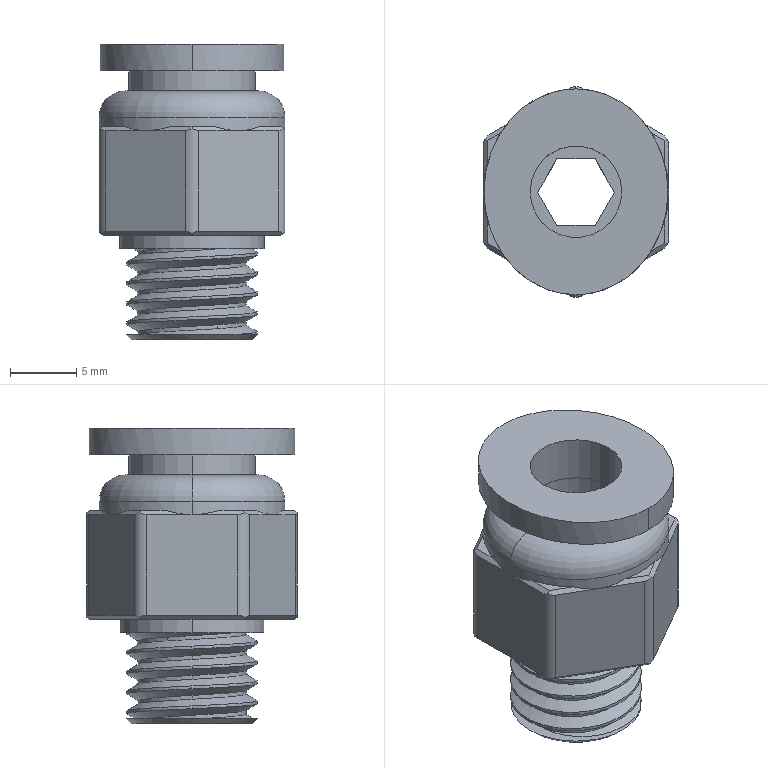Part | SolidWorks | features BaseBody 2 | 2 solids | 95 faces | box 14 x 15.856 x 22.23 mm | volume 1913 mm3 | plane 47 | cylinder 40 | spline 4 | torus 2 | cone 2 | commonest cylinder face diameters 8.141 x10 9.85 x10 2 x6 6.9 x4 6.84 x2 7.37 x2